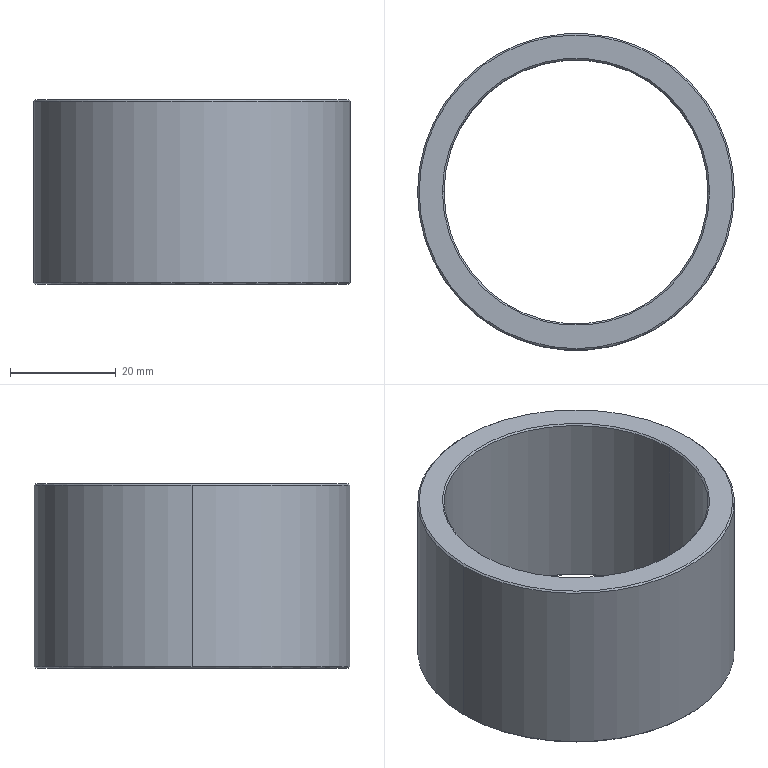Part | SolidWorks | features Chamfer 1, Extrusion 1 | 1 solid | 14 faces | box 60 x 60 x 35 mm | volume 30207 mm3 | cone 8 | cylinder 4 | plane 2 | commonest cylinder face diameters 50 x2 60 x2
STEP:
#1=CARTESIAN_POINT('',(-25.,0.,34.7));
#2=VERTEX_POINT('',#1);
#3=CARTESIAN_POINT('',(25.,0.,34.7));
#4=VERTEX_POINT('',#3);
#5=CARTESIAN_POINT('',(0.,0.,34.7));
#6=DIRECTION('',(0.,0.,1.));
#7=DIRECTION('',(1.,0.,0.));
#8=AXIS2_PLACEMENT_3D('',#5,#6,#7);
#9=CIRCLE('',#8,25.);
#10=EDGE_CURVE('',#2,#4,#9,.T.);
#11=ORIENTED_EDGE('',*,*,#10,.F.);
#12=CARTESIAN_POINT('',(-25.3,0.,35.));
#13=VERTEX_POINT('',#12);
#14=CARTESIAN_POINT('',(-25.,0.,34.7));
#15=DIRECTION('',(-0.7071,0.,0.7071));
#16=VECTOR('',#15,1000.);
#17=LINE('',#14,#16);
#18=EDGE_CURVE('',#2,#13,#17,.T.);
#19=ORIENTED_EDGE('',*,*,#18,.T.);
#20=CARTESIAN_POINT('',(25.3,0.,35.));
#21=VERTEX_POINT('',#20);
#22=CARTESIAN_POINT('',(0.,0.,35.));
#23=DIRECTION('',(0.,0.,-1.));
#24=DIRECTION('',(1.,0.,0.));
#25=AXIS2_PLACEMENT_3D('',#22,#23,#24);
#26=CIRCLE('',#25,25.3);
#27=EDGE_CURVE('',#21,#13,#26,.T.);
#28=ORIENTED_EDGE('',*,*,#27,.F.);
#29=CARTESIAN_POINT('',(25.,0.,34.7));
#30=DIRECTION('',(0.7071,0.,0.7071));
#31=VECTOR('',#30,1000.);
#32=LINE('',#29,#31);
#33=EDGE_CURVE('',#4,#21,#32,.T.);
#34=ORIENTED_EDGE('',*,*,#33,.F.);
#35=EDGE_LOOP('',(#11,#19,#28,#34));
#36=FACE_OUTER_BOUND('',#35,.T.);
#37=CARTESIAN_POINT('',(0.,0.,34.7));
#38=DIRECTION('',(0.,0.,1.));
#39=DIRECTION('',(1.,0.,0.));
#40=AXIS2_PLACEMENT_3D('',#37,#38,#39);
#41=CONICAL_SURFACE('',#40,25.,0.7854);
#42=ADVANCED_FACE('',(#36),#41,.F.);
#43=CARTESIAN_POINT('',(25.,0.,0.3));
#44=VERTEX_POINT('',#43);
#45=CARTESIAN_POINT('',(-25.,0.,0.3));
#46=VERTEX_POINT('',#45);
#47=CARTESIAN_POINT('',(0.,0.,0.3));
#48=DIRECTION('',(0.,0.,-1.));
#49=DIRECTION('',(1.,0.,0.));
#50=AXIS2_PLACEMENT_3D('',#47,#48,#49);
#51=CIRCLE('',#50,25.);
#52=EDGE_CURVE('',#44,#46,#51,.T.);
#53=ORIENTED_EDGE('',*,*,#52,.F.);
#54=CARTESIAN_POINT('',(25.3,0.,0.));
#55=VERTEX_POINT('',#54);
#56=CARTESIAN_POINT('',(25.3,0.,0.));
#57=DIRECTION('',(0.7071,0.,-0.7071));
#58=VECTOR('',#57,1000.);
#59=LINE('',#56,#58);
#60=EDGE_CURVE('',#44,#55,#59,.T.);
#61=ORIENTED_EDGE('',*,*,#60,.T.);
#62=CARTESIAN_POINT('',(-25.3,0.,0.));
#63=VERTEX_POINT('',#62);
#64=CARTESIAN_POINT('',(0.,0.,0.));
#65=DIRECTION('',(0.,0.,1.));
#66=DIRECTION('',(1.,0.,0.));
#67=AXIS2_PLACEMENT_3D('',#64,#65,#66);
#68=CIRCLE('',#67,25.3);
#69=EDGE_CURVE('',#63,#55,#68,.T.);
#70=ORIENTED_EDGE('',*,*,#69,.F.);
#71=CARTESIAN_POINT('',(-25.3,0.,0.));
#72=DIRECTION('',(-0.7071,0.,-0.7071));
#73=VECTOR('',#72,1000.);
#74=LINE('',#71,#73);
#75=EDGE_CURVE('',#46,#63,#74,.T.);
#76=ORIENTED_EDGE('',*,*,#75,.F.);
#77=EDGE_LOOP('',(#53,#61,#70,#76));
#78=FACE_OUTER_BOUND('',#77,.T.);
#79=CARTESIAN_POINT('',(0.,0.,0.));
#80=DIRECTION('',(0.,0.,-1.));
#81=DIRECTION('',(-1.,0.,0.));
#82=AXIS2_PLACEMENT_3D('',#79,#80,#81);
#83=CONICAL_SURFACE('',#82,25.3,0.7854);
#84=ADVANCED_FACE('',(#78),#83,.F.);
#85=CARTESIAN_POINT('',(29.7,0.,35.));
#86=VERTEX_POINT('',#85);
#87=CARTESIAN_POINT('',(-29.7,0.,35.));
#88=VERTEX_POINT('',#87);
#89=CARTESIAN_POINT('',(0.,0.,35.));
#90=DIRECTION('',(0.,0.,1.));
#91=DIRECTION('',(1.,0.,0.));
#92=AXIS2_PLACEMENT_3D('',#89,#90,#91);
#93=CIRCLE('',#92,29.7);
#94=EDGE_CURVE('',#86,#88,#93,.T.);
#95=ORIENTED_EDGE('',*,*,#94,.F.);
#96=CARTESIAN_POINT('',(30.,0.,34.7));
#97=VERTEX_POINT('',#96);
#98=CARTESIAN_POINT('',(29.7,0.,35.));
#99=DIRECTION('',(0.7071,0.,-0.7071));
#100=VECTOR('',#99,1000.);
#101=LINE('',#98,#100);
#102=EDGE_CURVE('',#86,#97,#101,.T.);
#103=ORIENTED_EDGE('',*,*,#102,.T.);
#104=CARTESIAN_POINT('',(-30.,0.,34.7));
#105=VERTEX_POINT('',#104);
#106=CARTESIAN_POINT('',(0.,0.,34.7));
#107=DIRECTION('',(0.,0.,-1.));
#108=DIRECTION('',(1.,0.,0.));
#109=AXIS2_PLACEMENT_3D('',#106,#107,#108);
#110=CIRCLE('',#109,30.);
#111=EDGE_CURVE('',#105,#97,#110,.T.);
#112=ORIENTED_EDGE('',*,*,#111,.F.);
#113=CARTESIAN_POINT('',(-29.7,0.,35.));
#114=DIRECTION('',(-0.7071,0.,-0.7071));
#115=VECTOR('',#114,1000.);
#116=LINE('',#113,#115);
#117=EDGE_CURVE('',#88,#105,#116,.T.);
#118=ORIENTED_EDGE('',*,*,#117,.F.);
#119=EDGE_LOOP('',(#95,#103,#112,#118));
#120=FACE_OUTER_BOUND('',#119,.T.);
#121=CARTESIAN_POINT('',(0.,0.,35.));
#122=DIRECTION('',(0.,0.,-1.));
#123=DIRECTION('',(-1.,0.,0.));
#124=AXIS2_PLACEMENT_3D('',#121,#122,#123);
#125=CONICAL_SURFACE('',#124,29.7,0.7854);
#126=ADVANCED_FACE('',(#120),#125,.T.);
#127=CARTESIAN_POINT('',(-29.7,0.,0.));
#128=VERTEX_POINT('',#127);
#129=CARTESIAN_POINT('',(29.7,0.,0.));
#130=VERTEX_POINT('',#129);
#131=CARTESIAN_POINT('',(0.,0.,0.));
#132=DIRECTION('',(0.,0.,-1.));
#133=DIRECTION('',(1.,0.,0.));
#134=AXIS2_PLACEMENT_3D('',#131,#132,#133);
#135=CIRCLE('',#134,29.7);
#136=EDGE_CURVE('',#128,#130,#135,.T.);
#137=ORIENTED_EDGE('',*,*,#136,.F.);
#138=CARTESIAN_POINT('',(-30.,0.,0.3));
#139=VERTEX_POINT('',#138);
#140=CARTESIAN_POINT('',(-30.,0.,0.3));
#141=DIRECTION('',(-0.7071,0.,0.7071));
#142=VECTOR('',#141,1000.);
#143=LINE('',#140,#142);
#144=EDGE_CURVE('',#128,#139,#143,.T.);
#145=ORIENTED_EDGE('',*,*,#144,.T.);
#146=CARTESIAN_POINT('',(30.,0.,0.3));
#147=VERTEX_POINT('',#146);
#148=CARTESIAN_POINT('',(0.,0.,0.3));
#149=DIRECTION('',(0.,0.,1.));
#150=DIRECTION('',(1.,0.,0.));
#151=AXIS2_PLACEMENT_3D('',#148,#149,#150);
#152=CIRCLE('',#151,30.);
#153=EDGE_CURVE('',#147,#139,#152,.T.);
#154=ORIENTED_EDGE('',*,*,#153,.F.);
#155=CARTESIAN_POINT('',(30.,0.,0.3));
#156=DIRECTION('',(0.7071,0.,0.7071));
#157=VECTOR('',#156,1000.);
#158=LINE('',#155,#157);
#159=EDGE_CURVE('',#130,#147,#158,.T.);
#160=ORIENTED_EDGE('',*,*,#159,.F.);
#161=EDGE_LOOP('',(#137,#145,#154,#160));
#162=FACE_OUTER_BOUND('',#161,.T.);
#163=CARTESIAN_POINT('',(0.,0.,0.3));
#164=DIRECTION('',(0.,0.,1.));
#165=DIRECTION('',(1.,0.,0.));
#166=AXIS2_PLACEMENT_3D('',#163,#164,#165);
#167=CONICAL_SURFACE('',#166,30.,0.7854);
#168=ADVANCED_FACE('',(#162),#167,.T.);
#169=ORIENTED_EDGE('',*,*,#10,.T.);
#170=CARTESIAN_POINT('',(25.,0.,35.));
#171=DIRECTION('',(0.,0.,-1.));
#172=VECTOR('',#171,1000.);
#173=LINE('',#170,#172);
#174=EDGE_CURVE('',#4,#44,#173,.T.);
#175=ORIENTED_EDGE('',*,*,#174,.T.);
#176=ORIENTED_EDGE('',*,*,#52,.T.);
#177=CARTESIAN_POINT('',(-25.,0.,35.));
#178=DIRECTION('',(0.,0.,-1.));
#179=VECTOR('',#178,1000.);
#180=LINE('',#177,#179);
#181=EDGE_CURVE('',#2,#46,#180,.T.);
#182=ORIENTED_EDGE('',*,*,#181,.F.);
#183=EDGE_LOOP('',(#169,#175,#176,#182));
#184=FACE_OUTER_BOUND('',#183,.T.);
#185=CARTESIAN_POINT('',(0.,0.,35.));
#186=DIRECTION('',(0.,0.,-1.));
#187=DIRECTION('',(-1.,0.,0.));
#188=AXIS2_PLACEMENT_3D('',#185,#186,#187);
#189=CYLINDRICAL_SURFACE('',#188,25.);
#190=ADVANCED_FACE('',(#184),#189,.F.);
#191=ORIENTED_EDGE('',*,*,#111,.T.);
#192=CARTESIAN_POINT('',(30.,0.,35.));
#193=DIRECTION('',(0.,0.,-1.));
#194=VECTOR('',#193,1000.);
#195=LINE('',#192,#194);
#196=EDGE_CURVE('',#97,#147,#195,.T.);
#197=ORIENTED_EDGE('',*,*,#196,.T.);
#198=ORIENTED_EDGE('',*,*,#153,.T.);
#199=CARTESIAN_POINT('',(-30.,0.,35.));
#200=DIRECTION('',(0.,0.,-1.));
#201=VECTOR('',#200,1000.);
#202=LINE('',#199,#201);
#203=EDGE_CURVE('',#105,#139,#202,.T.);
#204=ORIENTED_EDGE('',*,*,#203,.F.);
#205=EDGE_LOOP('',(#191,#197,#198,#204));
#206=FACE_OUTER_BOUND('',#205,.T.);
#207=CARTESIAN_POINT('',(0.,0.,35.));
#208=DIRECTION('',(0.,0.,-1.));
#209=DIRECTION('',(-1.,0.,0.));
#210=AXIS2_PLACEMENT_3D('',#207,#208,#209);
#211=CYLINDRICAL_SURFACE('',#210,30.);
#212=ADVANCED_FACE('',(#206),#211,.T.);
#213=CARTESIAN_POINT('',(0.,0.,35.));
#214=DIRECTION('',(0.,0.,1.));
#215=DIRECTION('',(1.,0.,0.));
#216=AXIS2_PLACEMENT_3D('',#213,#214,#215);
#217=CIRCLE('',#216,29.7);
#218=EDGE_CURVE('',#88,#86,#217,.T.);
#219=ORIENTED_EDGE('',*,*,#218,.T.);
#220=ORIENTED_EDGE('',*,*,#94,.T.);
#221=EDGE_LOOP('',(#219,#220));
#222=FACE_OUTER_BOUND('',#221,.T.);
#223=ORIENTED_EDGE('',*,*,#27,.T.);
#224=CARTESIAN_POINT('',(0.,0.,35.));
#225=DIRECTION('',(0.,0.,-1.));
#226=DIRECTION('',(1.,0.,0.));
#227=AXIS2_PLACEMENT_3D('',#224,#225,#226);
#228=CIRCLE('',#227,25.3);
#229=EDGE_CURVE('',#13,#21,#228,.T.);
#230=ORIENTED_EDGE('',*,*,#229,.T.);
#231=EDGE_LOOP('',(#223,#230));
#232=FACE_BOUND('',#231,.T.);
#233=CARTESIAN_POINT('',(0.,0.,35.));
#234=DIRECTION('',(0.,0.,1.));
#235=DIRECTION('',(1.,0.,0.));
#236=AXIS2_PLACEMENT_3D('',#233,#234,#235);
#237=PLANE('',#236);
#238=ADVANCED_FACE('',(#222,#232),#237,.T.);
#239=CARTESIAN_POINT('',(0.,0.,0.));
#240=DIRECTION('',(0.,0.,-1.));
#241=DIRECTION('',(1.,0.,0.));
#242=AXIS2_PLACEMENT_3D('',#239,#240,#241);
#243=CIRCLE('',#242,29.7);
#244=EDGE_CURVE('',#130,#128,#243,.T.);
#245=ORIENTED_EDGE('',*,*,#244,.T.);
#246=ORIENTED_EDGE('',*,*,#136,.T.);
#247=EDGE_LOOP('',(#245,#246));
#248=FACE_OUTER_BOUND('',#247,.T.);
#249=ORIENTED_EDGE('',*,*,#69,.T.);
#250=CARTESIAN_POINT('',(0.,0.,0.));
#251=DIRECTION('',(0.,0.,1.));
#252=DIRECTION('',(1.,0.,0.));
#253=AXIS2_PLACEMENT_3D('',#250,#251,#252);
#254=CIRCLE('',#253,25.3);
#255=EDGE_CURVE('',#55,#63,#254,.T.);
#256=ORIENTED_EDGE('',*,*,#255,.T.);
#257=EDGE_LOOP('',(#249,#256));
#258=FACE_BOUND('',#257,.T.);
#259=CARTESIAN_POINT('',(0.,0.,0.));
#260=DIRECTION('',(0.,0.,1.));
#261=DIRECTION('',(1.,0.,0.));
#262=AXIS2_PLACEMENT_3D('',#259,#260,#261);
#263=PLANE('',#262);
#264=ADVANCED_FACE('',(#248,#258),#263,.F.);
#265=ORIENTED_EDGE('',*,*,#196,.F.);
#266=CARTESIAN_POINT('',(0.,0.,34.7));
#267=DIRECTION('',(0.,0.,-1.));
#268=DIRECTION('',(1.,0.,0.));
#269=AXIS2_PLACEMENT_3D('',#266,#267,#268);
#270=CIRCLE('',#269,30.);
#271=EDGE_CURVE('',#97,#105,#270,.T.);
#272=ORIENTED_EDGE('',*,*,#271,.T.);
#273=ORIENTED_EDGE('',*,*,#203,.T.);
#274=CARTESIAN_POINT('',(0.,0.,0.3));
#275=DIRECTION('',(0.,0.,1.));
#276=DIRECTION('',(1.,0.,0.));
#277=AXIS2_PLACEMENT_3D('',#274,#275,#276);
#278=CIRCLE('',#277,30.);
#279=EDGE_CURVE('',#139,#147,#278,.T.);
#280=ORIENTED_EDGE('',*,*,#279,.T.);
#281=EDGE_LOOP('',(#265,#272,#273,#280));
#282=FACE_OUTER_BOUND('',#281,.T.);
#283=CARTESIAN_POINT('',(0.,0.,35.));
#284=DIRECTION('',(0.,0.,-1.));
#285=DIRECTION('',(-1.,0.,0.));
#286=AXIS2_PLACEMENT_3D('',#283,#284,#285);
#287=CYLINDRICAL_SURFACE('',#286,30.);
#288=ADVANCED_FACE('',(#282),#287,.T.);
#289=ORIENTED_EDGE('',*,*,#174,.F.);
#290=CARTESIAN_POINT('',(0.,0.,34.7));
#291=DIRECTION('',(0.,0.,1.));
#292=DIRECTION('',(1.,0.,0.));
#293=AXIS2_PLACEMENT_3D('',#290,#291,#292);
#294=CIRCLE('',#293,25.);
#295=EDGE_CURVE('',#4,#2,#294,.T.);
#296=ORIENTED_EDGE('',*,*,#295,.T.);
#297=ORIENTED_EDGE('',*,*,#181,.T.);
#298=CARTESIAN_POINT('',(0.,0.,0.3));
#299=DIRECTION('',(0.,0.,-1.));
#300=DIRECTION('',(1.,0.,0.));
#301=AXIS2_PLACEMENT_3D('',#298,#299,#300);
#302=CIRCLE('',#301,25.);
#303=EDGE_CURVE('',#46,#44,#302,.T.);
#304=ORIENTED_EDGE('',*,*,#303,.T.);
#305=EDGE_LOOP('',(#289,#296,#297,#304));
#306=FACE_OUTER_BOUND('',#305,.T.);
#307=CARTESIAN_POINT('',(0.,0.,35.));
#308=DIRECTION('',(0.,0.,-1.));
#309=DIRECTION('',(-1.,0.,0.));
#310=AXIS2_PLACEMENT_3D('',#307,#308,#309);
#311=CYLINDRICAL_SURFACE('',#310,25.);
#312=ADVANCED_FACE('',(#306),#311,.F.);
#313=ORIENTED_EDGE('',*,*,#144,.F.);
#314=ORIENTED_EDGE('',*,*,#244,.F.);
#315=ORIENTED_EDGE('',*,*,#159,.T.);
#316=ORIENTED_EDGE('',*,*,#279,.F.);
#317=EDGE_LOOP('',(#313,#314,#315,#316));
#318=FACE_OUTER_BOUND('',#317,.T.);
#319=CARTESIAN_POINT('',(0.,0.,0.3));
#320=DIRECTION('',(0.,0.,1.));
#321=DIRECTION('',(1.,0.,0.));
#322=AXIS2_PLACEMENT_3D('',#319,#320,#321);
#323=CONICAL_SURFACE('',#322,30.,0.7854);
#324=ADVANCED_FACE('',(#318),#323,.T.);
#325=ORIENTED_EDGE('',*,*,#102,.F.);
#326=ORIENTED_EDGE('',*,*,#218,.F.);
#327=ORIENTED_EDGE('',*,*,#117,.T.);
#328=ORIENTED_EDGE('',*,*,#271,.F.);
#329=EDGE_LOOP('',(#325,#326,#327,#328));
#330=FACE_OUTER_BOUND('',#329,.T.);
#331=CARTESIAN_POINT('',(0.,0.,35.));
#332=DIRECTION('',(0.,0.,-1.));
#333=DIRECTION('',(-1.,0.,0.));
#334=AXIS2_PLACEMENT_3D('',#331,#332,#333);
#335=CONICAL_SURFACE('',#334,29.7,0.7854);
#336=ADVANCED_FACE('',(#330),#335,.T.);
#337=ORIENTED_EDGE('',*,*,#60,.F.);
#338=ORIENTED_EDGE('',*,*,#303,.F.);
#339=ORIENTED_EDGE('',*,*,#75,.T.);
#340=ORIENTED_EDGE('',*,*,#255,.F.);
#341=EDGE_LOOP('',(#337,#338,#339,#340));
#342=FACE_OUTER_BOUND('',#341,.T.);
#343=CARTESIAN_POINT('',(0.,0.,0.));
#344=DIRECTION('',(0.,0.,-1.));
#345=DIRECTION('',(-1.,0.,0.));
#346=AXIS2_PLACEMENT_3D('',#343,#344,#345);
#347=CONICAL_SURFACE('',#346,25.3,0.7854);
#348=ADVANCED_FACE('',(#342),#347,.F.);
#349=ORIENTED_EDGE('',*,*,#18,.F.);
#350=ORIENTED_EDGE('',*,*,#295,.F.);
#351=ORIENTED_EDGE('',*,*,#33,.T.);
#352=ORIENTED_EDGE('',*,*,#229,.F.);
#353=EDGE_LOOP('',(#349,#350,#351,#352));
#354=FACE_OUTER_BOUND('',#353,.T.);
#355=CARTESIAN_POINT('',(0.,0.,34.7));
#356=DIRECTION('',(0.,0.,1.));
#357=DIRECTION('',(1.,0.,0.));
#358=AXIS2_PLACEMENT_3D('',#355,#356,#357);
#359=CONICAL_SURFACE('',#358,25.,0.7854);
#360=ADVANCED_FACE('',(#354),#359,.F.);
#361=CLOSED_SHELL('',(#42,#84,#126,#168,#190,#212,#238,#264,#288,#312,#324,#336,#348,#360));
#362=MANIFOLD_SOLID_BREP('',#361);
#363=CARTESIAN_POINT('',(0.,0.,0.));
#364=DIRECTION('',(0.,0.,1.));
#365=DIRECTION('',(1.,0.,0.));
#366=AXIS2_PLACEMENT_3D('',#363,#364,#365);
#367=(LENGTH_UNIT()NAMED_UNIT(*)SI_UNIT(.MILLI.,.METRE.));
#368=UNCERTAINTY_MEASURE_WITH_UNIT(LENGTH_MEASURE(0.00001),#367,'','');
#369=(NAMED_UNIT(*)PLANE_ANGLE_UNIT()SI_UNIT($,.RADIAN.));
#370=(NAMED_UNIT(*)SI_UNIT($,.STERADIAN.)SOLID_ANGLE_UNIT());
#371=(GEOMETRIC_REPRESENTATION_CONTEXT(3)GLOBAL_UNCERTAINTY_ASSIGNED_CONTEXT((#368))GLOBAL_UNIT_ASSIGNED_CONTEXT((#367,#369,#370))REPRESENTATION_CONTEXT('',''));
#372=ADVANCED_BREP_SHAPE_REPRESENTATION('',(#362,#366),#371);